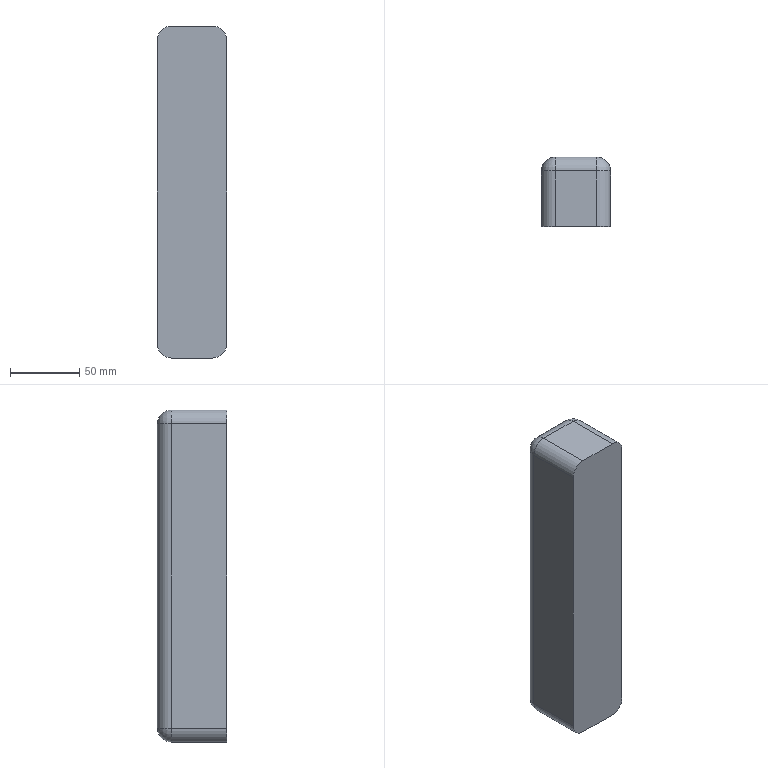Part | SolidWorks | features ICE 2, Extrusion 1, Fillet 1 | 1 solid | 18 faces | box 50 x 50 x 240 mm | volume 583931 mm3 | cylinder 8 | plane 6 | sphere 4 | commonest cylinder face diameters 20 x8
STEP:
#1=CARTESIAN_POINT('',(0.,40.,10.));
#2=VERTEX_POINT('',#1);
#3=CARTESIAN_POINT('',(0.,0.,10.));
#4=VERTEX_POINT('',#3);
#5=CARTESIAN_POINT('',(0.,0.,10.));
#6=DIRECTION('',(0.,-1.,0.));
#7=VECTOR('',#6,1000.);
#8=LINE('',#5,#7);
#9=EDGE_CURVE('',#2,#4,#8,.T.);
#10=ORIENTED_EDGE('',*,*,#9,.T.);
#11=CARTESIAN_POINT('',(0.,0.,230.));
#12=VERTEX_POINT('',#11);
#13=CARTESIAN_POINT('',(0.,0.,290.));
#14=DIRECTION('',(0.,0.,-1.));
#15=VECTOR('',#14,1000.);
#16=LINE('',#13,#15);
#17=EDGE_CURVE('',#12,#4,#16,.T.);
#18=ORIENTED_EDGE('',*,*,#17,.F.);
#19=CARTESIAN_POINT('',(0.,40.,230.));
#20=VERTEX_POINT('',#19);
#21=CARTESIAN_POINT('',(0.,50.,230.));
#22=DIRECTION('',(0.,1.,0.));
#23=VECTOR('',#22,1000.);
#24=LINE('',#21,#23);
#25=EDGE_CURVE('',#12,#20,#24,.T.);
#26=ORIENTED_EDGE('',*,*,#25,.T.);
#27=CARTESIAN_POINT('',(0.,40.,240.));
#28=DIRECTION('',(0.,0.,-1.));
#29=VECTOR('',#28,1000.);
#30=LINE('',#27,#29);
#31=EDGE_CURVE('',#20,#2,#30,.T.);
#32=ORIENTED_EDGE('',*,*,#31,.T.);
#33=EDGE_LOOP('',(#10,#18,#26,#32));
#34=FACE_OUTER_BOUND('',#33,.T.);
#35=CARTESIAN_POINT('',(0.,0.,240.));
#36=DIRECTION('',(1.,0.,0.));
#37=DIRECTION('',(0.,0.,-1.));
#38=AXIS2_PLACEMENT_3D('',#35,#36,#37);
#39=PLANE('',#38);
#40=ADVANCED_FACE('',(#34),#39,.F.);
#41=CARTESIAN_POINT('',(50.,40.,230.));
#42=VERTEX_POINT('',#41);
#43=CARTESIAN_POINT('',(50.,0.,230.));
#44=VERTEX_POINT('',#43);
#45=CARTESIAN_POINT('',(50.,0.,230.));
#46=DIRECTION('',(0.,-1.,0.));
#47=VECTOR('',#46,1000.);
#48=LINE('',#45,#47);
#49=EDGE_CURVE('',#42,#44,#48,.T.);
#50=ORIENTED_EDGE('',*,*,#49,.T.);
#51=CARTESIAN_POINT('',(50.,0.,10.));
#52=VERTEX_POINT('',#51);
#53=CARTESIAN_POINT('',(50.,0.,240.));
#54=DIRECTION('',(0.,0.,-1.));
#55=VECTOR('',#54,1000.);
#56=LINE('',#53,#55);
#57=EDGE_CURVE('',#44,#52,#56,.T.);
#58=ORIENTED_EDGE('',*,*,#57,.T.);
#59=CARTESIAN_POINT('',(50.,40.,10.));
#60=VERTEX_POINT('',#59);
#61=CARTESIAN_POINT('',(50.,0.,10.));
#62=DIRECTION('',(0.,1.,0.));
#63=VECTOR('',#62,1000.);
#64=LINE('',#61,#63);
#65=EDGE_CURVE('',#52,#60,#64,.T.);
#66=ORIENTED_EDGE('',*,*,#65,.T.);
#67=CARTESIAN_POINT('',(50.,40.,240.));
#68=DIRECTION('',(0.,0.,1.));
#69=VECTOR('',#68,1000.);
#70=LINE('',#67,#69);
#71=EDGE_CURVE('',#60,#42,#70,.T.);
#72=ORIENTED_EDGE('',*,*,#71,.T.);
#73=EDGE_LOOP('',(#50,#58,#66,#72));
#74=FACE_OUTER_BOUND('',#73,.T.);
#75=CARTESIAN_POINT('',(50.,0.,240.));
#76=DIRECTION('',(-1.,0.,0.));
#77=DIRECTION('',(0.,0.,1.));
#78=AXIS2_PLACEMENT_3D('',#75,#76,#77);
#79=PLANE('',#78);
#80=ADVANCED_FACE('',(#74),#79,.F.);
#81=CARTESIAN_POINT('',(10.,50.,10.));
#82=VERTEX_POINT('',#81);
#83=CARTESIAN_POINT('',(10.,50.,230.));
#84=VERTEX_POINT('',#83);
#85=CARTESIAN_POINT('',(10.,50.,240.));
#86=DIRECTION('',(0.,0.,1.));
#87=VECTOR('',#86,1000.);
#88=LINE('',#85,#87);
#89=EDGE_CURVE('',#82,#84,#88,.T.);
#90=ORIENTED_EDGE('',*,*,#89,.T.);
#91=CARTESIAN_POINT('',(40.,50.,230.));
#92=VERTEX_POINT('',#91);
#93=CARTESIAN_POINT('',(50.,50.,230.));
#94=DIRECTION('',(1.,0.,0.));
#95=VECTOR('',#94,1000.);
#96=LINE('',#93,#95);
#97=EDGE_CURVE('',#84,#92,#96,.T.);
#98=ORIENTED_EDGE('',*,*,#97,.T.);
#99=CARTESIAN_POINT('',(40.,50.,10.));
#100=VERTEX_POINT('',#99);
#101=CARTESIAN_POINT('',(40.,50.,240.));
#102=DIRECTION('',(0.,0.,-1.));
#103=VECTOR('',#102,1000.);
#104=LINE('',#101,#103);
#105=EDGE_CURVE('',#92,#100,#104,.T.);
#106=ORIENTED_EDGE('',*,*,#105,.T.);
#107=CARTESIAN_POINT('',(50.,50.,10.));
#108=DIRECTION('',(-1.,0.,0.));
#109=VECTOR('',#108,1000.);
#110=LINE('',#107,#109);
#111=EDGE_CURVE('',#100,#82,#110,.T.);
#112=ORIENTED_EDGE('',*,*,#111,.T.);
#113=EDGE_LOOP('',(#90,#98,#106,#112));
#114=FACE_OUTER_BOUND('',#113,.T.);
#115=CARTESIAN_POINT('',(50.,50.,240.));
#116=DIRECTION('',(0.,-1.,0.));
#117=DIRECTION('',(0.,0.,-1.));
#118=AXIS2_PLACEMENT_3D('',#115,#116,#117);
#119=PLANE('',#118);
#120=ADVANCED_FACE('',(#114),#119,.F.);
#121=CARTESIAN_POINT('',(40.,40.,240.));
#122=VERTEX_POINT('',#121);
#123=CARTESIAN_POINT('',(10.,40.,240.));
#124=VERTEX_POINT('',#123);
#125=CARTESIAN_POINT('',(0.,40.,240.));
#126=DIRECTION('',(-1.,0.,0.));
#127=VECTOR('',#126,1000.);
#128=LINE('',#125,#127);
#129=EDGE_CURVE('',#122,#124,#128,.T.);
#130=ORIENTED_EDGE('',*,*,#129,.T.);
#131=CARTESIAN_POINT('',(10.,0.,240.));
#132=VERTEX_POINT('',#131);
#133=CARTESIAN_POINT('',(10.,0.,240.));
#134=DIRECTION('',(0.,-1.,0.));
#135=VECTOR('',#134,1000.);
#136=LINE('',#133,#135);
#137=EDGE_CURVE('',#124,#132,#136,.T.);
#138=ORIENTED_EDGE('',*,*,#137,.T.);
#139=CARTESIAN_POINT('',(40.,0.,240.));
#140=VERTEX_POINT('',#139);
#141=CARTESIAN_POINT('',(0.,0.,240.));
#142=DIRECTION('',(1.,0.,0.));
#143=VECTOR('',#142,1000.);
#144=LINE('',#141,#143);
#145=EDGE_CURVE('',#132,#140,#144,.T.);
#146=ORIENTED_EDGE('',*,*,#145,.T.);
#147=CARTESIAN_POINT('',(40.,50.,240.));
#148=DIRECTION('',(0.,1.,0.));
#149=VECTOR('',#148,1000.);
#150=LINE('',#147,#149);
#151=EDGE_CURVE('',#140,#122,#150,.T.);
#152=ORIENTED_EDGE('',*,*,#151,.T.);
#153=EDGE_LOOP('',(#130,#138,#146,#152));
#154=FACE_OUTER_BOUND('',#153,.T.);
#155=CARTESIAN_POINT('',(0.,0.,240.));
#156=DIRECTION('',(0.,0.,1.));
#157=DIRECTION('',(1.,0.,0.));
#158=AXIS2_PLACEMENT_3D('',#155,#156,#157);
#159=PLANE('',#158);
#160=ADVANCED_FACE('',(#154),#159,.T.);
#161=CARTESIAN_POINT('',(10.,40.,0.));
#162=VERTEX_POINT('',#161);
#163=CARTESIAN_POINT('',(40.,40.,0.));
#164=VERTEX_POINT('',#163);
#165=CARTESIAN_POINT('',(0.,40.,0.));
#166=DIRECTION('',(1.,0.,0.));
#167=VECTOR('',#166,1000.);
#168=LINE('',#165,#167);
#169=EDGE_CURVE('',#162,#164,#168,.T.);
#170=ORIENTED_EDGE('',*,*,#169,.T.);
#171=CARTESIAN_POINT('',(40.,0.,0.));
#172=VERTEX_POINT('',#171);
#173=CARTESIAN_POINT('',(40.,0.,0.));
#174=DIRECTION('',(0.,-1.,0.));
#175=VECTOR('',#174,1000.);
#176=LINE('',#173,#175);
#177=EDGE_CURVE('',#164,#172,#176,.T.);
#178=ORIENTED_EDGE('',*,*,#177,.T.);
#179=CARTESIAN_POINT('',(10.,0.,0.));
#180=VERTEX_POINT('',#179);
#181=CARTESIAN_POINT('',(0.,0.,0.));
#182=DIRECTION('',(1.,0.,0.));
#183=VECTOR('',#182,1000.);
#184=LINE('',#181,#183);
#185=EDGE_CURVE('',#180,#172,#184,.T.);
#186=ORIENTED_EDGE('',*,*,#185,.F.);
#187=CARTESIAN_POINT('',(10.,0.,0.));
#188=DIRECTION('',(0.,1.,0.));
#189=VECTOR('',#188,1000.);
#190=LINE('',#187,#189);
#191=EDGE_CURVE('',#180,#162,#190,.T.);
#192=ORIENTED_EDGE('',*,*,#191,.T.);
#193=EDGE_LOOP('',(#170,#178,#186,#192));
#194=FACE_OUTER_BOUND('',#193,.T.);
#195=CARTESIAN_POINT('',(0.,0.,0.));
#196=DIRECTION('',(0.,0.,1.));
#197=DIRECTION('',(1.,0.,0.));
#198=AXIS2_PLACEMENT_3D('',#195,#196,#197);
#199=PLANE('',#198);
#200=ADVANCED_FACE('',(#194),#199,.F.);
#201=CARTESIAN_POINT('',(40.,0.,10.));
#202=DIRECTION('',(0.,-1.,0.));
#203=DIRECTION('',(0.,0.,1.));
#204=AXIS2_PLACEMENT_3D('',#201,#202,#203);
#205=CIRCLE('',#204,10.);
#206=EDGE_CURVE('',#172,#52,#205,.T.);
#207=ORIENTED_EDGE('',*,*,#206,.F.);
#208=ORIENTED_EDGE('',*,*,#177,.F.);
#209=CARTESIAN_POINT('',(40.,40.,10.));
#210=DIRECTION('',(0.,1.,0.));
#211=DIRECTION('',(0.,0.,1.));
#212=AXIS2_PLACEMENT_3D('',#209,#210,#211);
#213=CIRCLE('',#212,10.);
#214=EDGE_CURVE('',#60,#164,#213,.T.);
#215=ORIENTED_EDGE('',*,*,#214,.F.);
#216=ORIENTED_EDGE('',*,*,#65,.F.);
#217=EDGE_LOOP('',(#207,#208,#215,#216));
#218=FACE_OUTER_BOUND('',#217,.T.);
#219=CARTESIAN_POINT('',(40.,0.,10.));
#220=DIRECTION('',(0.,1.,0.));
#221=DIRECTION('',(0.,0.,1.));
#222=AXIS2_PLACEMENT_3D('',#219,#220,#221);
#223=CYLINDRICAL_SURFACE('',#222,10.);
#224=ADVANCED_FACE('',(#218),#223,.T.);
#225=CARTESIAN_POINT('',(10.,0.,10.));
#226=DIRECTION('',(0.,-1.,0.));
#227=DIRECTION('',(0.,0.,1.));
#228=AXIS2_PLACEMENT_3D('',#225,#226,#227);
#229=CIRCLE('',#228,10.);
#230=EDGE_CURVE('',#4,#180,#229,.T.);
#231=ORIENTED_EDGE('',*,*,#230,.F.);
#232=ORIENTED_EDGE('',*,*,#9,.F.);
#233=CARTESIAN_POINT('',(10.,40.,10.));
#234=DIRECTION('',(0.,1.,0.));
#235=DIRECTION('',(0.,0.,1.));
#236=AXIS2_PLACEMENT_3D('',#233,#234,#235);
#237=CIRCLE('',#236,10.);
#238=EDGE_CURVE('',#162,#2,#237,.T.);
#239=ORIENTED_EDGE('',*,*,#238,.F.);
#240=ORIENTED_EDGE('',*,*,#191,.F.);
#241=EDGE_LOOP('',(#231,#232,#239,#240));
#242=FACE_OUTER_BOUND('',#241,.T.);
#243=CARTESIAN_POINT('',(10.,0.,10.));
#244=DIRECTION('',(0.,-1.,0.));
#245=DIRECTION('',(0.,0.,-1.));
#246=AXIS2_PLACEMENT_3D('',#243,#244,#245);
#247=CYLINDRICAL_SURFACE('',#246,10.);
#248=ADVANCED_FACE('',(#242),#247,.T.);
#249=CARTESIAN_POINT('',(40.,40.,10.));
#250=DIRECTION('',(1.,0.,0.));
#251=DIRECTION('',(0.,0.,-1.));
#252=AXIS2_PLACEMENT_3D('',#249,#250,#251);
#253=CIRCLE('',#252,10.);
#254=EDGE_CURVE('',#164,#100,#253,.T.);
#255=ORIENTED_EDGE('',*,*,#254,.F.);
#256=ORIENTED_EDGE('',*,*,#169,.F.);
#257=CARTESIAN_POINT('',(10.,40.,10.));
#258=DIRECTION('',(-1.,0.,0.));
#259=DIRECTION('',(0.,0.,1.));
#260=AXIS2_PLACEMENT_3D('',#257,#258,#259);
#261=CIRCLE('',#260,10.);
#262=EDGE_CURVE('',#82,#162,#261,.T.);
#263=ORIENTED_EDGE('',*,*,#262,.F.);
#264=ORIENTED_EDGE('',*,*,#111,.F.);
#265=EDGE_LOOP('',(#255,#256,#263,#264));
#266=FACE_OUTER_BOUND('',#265,.T.);
#267=CARTESIAN_POINT('',(50.,40.,10.));
#268=DIRECTION('',(-1.,0.,0.));
#269=DIRECTION('',(0.,0.,1.));
#270=AXIS2_PLACEMENT_3D('',#267,#268,#269);
#271=CYLINDRICAL_SURFACE('',#270,10.);
#272=ADVANCED_FACE('',(#266),#271,.T.);
#273=ORIENTED_EDGE('',*,*,#214,.T.);
#274=ORIENTED_EDGE('',*,*,#254,.T.);
#275=CARTESIAN_POINT('',(40.,40.,10.));
#276=DIRECTION('',(0.,0.,1.));
#277=DIRECTION('',(-1.,0.,0.));
#278=AXIS2_PLACEMENT_3D('',#275,#276,#277);
#279=CIRCLE('',#278,10.);
#280=EDGE_CURVE('',#60,#100,#279,.T.);
#281=ORIENTED_EDGE('',*,*,#280,.F.);
#282=EDGE_LOOP('',(#273,#274,#281));
#283=FACE_OUTER_BOUND('',#282,.T.);
#284=CARTESIAN_POINT('',(40.,40.,10.));
#285=DIRECTION('',(0.,1.,0.));
#286=DIRECTION('',(1.,0.,0.));
#287=AXIS2_PLACEMENT_3D('',#284,#285,#286);
#288=SPHERICAL_SURFACE('',#287,10.);
#289=ADVANCED_FACE('',(#283),#288,.T.);
#290=ORIENTED_EDGE('',*,*,#262,.T.);
#291=ORIENTED_EDGE('',*,*,#238,.T.);
#292=CARTESIAN_POINT('',(10.,40.,10.));
#293=DIRECTION('',(0.,0.,1.));
#294=DIRECTION('',(-1.,0.,0.));
#295=AXIS2_PLACEMENT_3D('',#292,#293,#294);
#296=CIRCLE('',#295,10.);
#297=EDGE_CURVE('',#82,#2,#296,.T.);
#298=ORIENTED_EDGE('',*,*,#297,.F.);
#299=EDGE_LOOP('',(#290,#291,#298));
#300=FACE_OUTER_BOUND('',#299,.T.);
#301=CARTESIAN_POINT('',(10.,40.,10.));
#302=DIRECTION('',(0.,1.,0.));
#303=DIRECTION('',(1.,0.,0.));
#304=AXIS2_PLACEMENT_3D('',#301,#302,#303);
#305=SPHERICAL_SURFACE('',#304,10.);
#306=ADVANCED_FACE('',(#300),#305,.T.);
#307=ORIENTED_EDGE('',*,*,#280,.T.);
#308=ORIENTED_EDGE('',*,*,#105,.F.);
#309=CARTESIAN_POINT('',(40.,40.,230.));
#310=DIRECTION('',(0.,0.,1.));
#311=DIRECTION('',(1.,0.,0.));
#312=AXIS2_PLACEMENT_3D('',#309,#310,#311);
#313=CIRCLE('',#312,10.);
#314=EDGE_CURVE('',#42,#92,#313,.T.);
#315=ORIENTED_EDGE('',*,*,#314,.F.);
#316=ORIENTED_EDGE('',*,*,#71,.F.);
#317=EDGE_LOOP('',(#307,#308,#315,#316));
#318=FACE_OUTER_BOUND('',#317,.T.);
#319=CARTESIAN_POINT('',(40.,40.,240.));
#320=DIRECTION('',(0.,0.,-1.));
#321=DIRECTION('',(-1.,0.,0.));
#322=AXIS2_PLACEMENT_3D('',#319,#320,#321);
#323=CYLINDRICAL_SURFACE('',#322,10.);
#324=ADVANCED_FACE('',(#318),#323,.T.);
#325=CARTESIAN_POINT('',(40.,0.,230.));
#326=DIRECTION('',(0.,-1.,0.));
#327=DIRECTION('',(0.,0.,1.));
#328=AXIS2_PLACEMENT_3D('',#325,#326,#327);
#329=CIRCLE('',#328,10.);
#330=EDGE_CURVE('',#44,#140,#329,.T.);
#331=ORIENTED_EDGE('',*,*,#330,.F.);
#332=ORIENTED_EDGE('',*,*,#49,.F.);
#333=CARTESIAN_POINT('',(40.,40.,230.));
#334=DIRECTION('',(0.,1.,0.));
#335=DIRECTION('',(0.,0.,1.));
#336=AXIS2_PLACEMENT_3D('',#333,#334,#335);
#337=CIRCLE('',#336,10.);
#338=EDGE_CURVE('',#122,#42,#337,.T.);
#339=ORIENTED_EDGE('',*,*,#338,.F.);
#340=ORIENTED_EDGE('',*,*,#151,.F.);
#341=EDGE_LOOP('',(#331,#332,#339,#340));
#342=FACE_OUTER_BOUND('',#341,.T.);
#343=CARTESIAN_POINT('',(40.,0.,230.));
#344=DIRECTION('',(0.,-1.,0.));
#345=DIRECTION('',(0.,0.,-1.));
#346=AXIS2_PLACEMENT_3D('',#343,#344,#345);
#347=CYLINDRICAL_SURFACE('',#346,10.);
#348=ADVANCED_FACE('',(#342),#347,.T.);
#349=CARTESIAN_POINT('',(10.,0.,230.));
#350=DIRECTION('',(0.,-1.,0.));
#351=DIRECTION('',(0.,0.,1.));
#352=AXIS2_PLACEMENT_3D('',#349,#350,#351);
#353=CIRCLE('',#352,10.);
#354=EDGE_CURVE('',#132,#12,#353,.T.);
#355=ORIENTED_EDGE('',*,*,#354,.F.);
#356=ORIENTED_EDGE('',*,*,#137,.F.);
#357=CARTESIAN_POINT('',(10.,40.,230.));
#358=DIRECTION('',(0.,1.,0.));
#359=DIRECTION('',(0.,0.,1.));
#360=AXIS2_PLACEMENT_3D('',#357,#358,#359);
#361=CIRCLE('',#360,10.);
#362=EDGE_CURVE('',#20,#124,#361,.T.);
#363=ORIENTED_EDGE('',*,*,#362,.F.);
#364=ORIENTED_EDGE('',*,*,#25,.F.);
#365=EDGE_LOOP('',(#355,#356,#363,#364));
#366=FACE_OUTER_BOUND('',#365,.T.);
#367=CARTESIAN_POINT('',(10.,0.,230.));
#368=DIRECTION('',(0.,1.,0.));
#369=DIRECTION('',(0.,0.,1.));
#370=AXIS2_PLACEMENT_3D('',#367,#368,#369);
#371=CYLINDRICAL_SURFACE('',#370,10.);
#372=ADVANCED_FACE('',(#366),#371,.T.);
#373=ORIENTED_EDGE('',*,*,#297,.T.);
#374=ORIENTED_EDGE('',*,*,#31,.F.);
#375=CARTESIAN_POINT('',(10.,40.,230.));
#376=DIRECTION('',(0.,0.,1.));
#377=DIRECTION('',(1.,0.,0.));
#378=AXIS2_PLACEMENT_3D('',#375,#376,#377);
#379=CIRCLE('',#378,10.);
#380=EDGE_CURVE('',#84,#20,#379,.T.);
#381=ORIENTED_EDGE('',*,*,#380,.F.);
#382=ORIENTED_EDGE('',*,*,#89,.F.);
#383=EDGE_LOOP('',(#373,#374,#381,#382));
#384=FACE_OUTER_BOUND('',#383,.T.);
#385=CARTESIAN_POINT('',(10.,40.,240.));
#386=DIRECTION('',(0.,0.,-1.));
#387=DIRECTION('',(-1.,0.,0.));
#388=AXIS2_PLACEMENT_3D('',#385,#386,#387);
#389=CYLINDRICAL_SURFACE('',#388,10.);
#390=ADVANCED_FACE('',(#384),#389,.T.);
#391=ORIENTED_EDGE('',*,*,#338,.T.);
#392=ORIENTED_EDGE('',*,*,#314,.T.);
#393=CARTESIAN_POINT('',(40.,40.,230.));
#394=DIRECTION('',(-1.,0.,0.));
#395=DIRECTION('',(0.,0.,-1.));
#396=AXIS2_PLACEMENT_3D('',#393,#394,#395);
#397=CIRCLE('',#396,10.);
#398=EDGE_CURVE('',#122,#92,#397,.T.);
#399=ORIENTED_EDGE('',*,*,#398,.F.);
#400=EDGE_LOOP('',(#391,#392,#399));
#401=FACE_OUTER_BOUND('',#400,.T.);
#402=CARTESIAN_POINT('',(40.,40.,230.));
#403=DIRECTION('',(0.,1.,0.));
#404=DIRECTION('',(1.,0.,0.));
#405=AXIS2_PLACEMENT_3D('',#402,#403,#404);
#406=SPHERICAL_SURFACE('',#405,10.);
#407=ADVANCED_FACE('',(#401),#406,.T.);
#408=ORIENTED_EDGE('',*,*,#380,.T.);
#409=ORIENTED_EDGE('',*,*,#362,.T.);
#410=CARTESIAN_POINT('',(10.,40.,230.));
#411=DIRECTION('',(1.,0.,0.));
#412=DIRECTION('',(0.,0.,1.));
#413=AXIS2_PLACEMENT_3D('',#410,#411,#412);
#414=CIRCLE('',#413,10.);
#415=EDGE_CURVE('',#84,#124,#414,.T.);
#416=ORIENTED_EDGE('',*,*,#415,.F.);
#417=EDGE_LOOP('',(#408,#409,#416));
#418=FACE_OUTER_BOUND('',#417,.T.);
#419=CARTESIAN_POINT('',(10.,40.,230.));
#420=DIRECTION('',(0.,1.,0.));
#421=DIRECTION('',(1.,0.,0.));
#422=AXIS2_PLACEMENT_3D('',#419,#420,#421);
#423=SPHERICAL_SURFACE('',#422,10.);
#424=ADVANCED_FACE('',(#418),#423,.T.);
#425=ORIENTED_EDGE('',*,*,#398,.T.);
#426=ORIENTED_EDGE('',*,*,#97,.F.);
#427=ORIENTED_EDGE('',*,*,#415,.T.);
#428=ORIENTED_EDGE('',*,*,#129,.F.);
#429=EDGE_LOOP('',(#425,#426,#427,#428));
#430=FACE_OUTER_BOUND('',#429,.T.);
#431=CARTESIAN_POINT('',(0.,40.,230.));
#432=DIRECTION('',(1.,0.,0.));
#433=DIRECTION('',(0.,0.,-1.));
#434=AXIS2_PLACEMENT_3D('',#431,#432,#433);
#435=CYLINDRICAL_SURFACE('',#434,10.);
#436=ADVANCED_FACE('',(#430),#435,.T.);
#437=ORIENTED_EDGE('',*,*,#230,.T.);
#438=ORIENTED_EDGE('',*,*,#185,.T.);
#439=ORIENTED_EDGE('',*,*,#206,.T.);
#440=ORIENTED_EDGE('',*,*,#57,.F.);
#441=ORIENTED_EDGE('',*,*,#330,.T.);
#442=ORIENTED_EDGE('',*,*,#145,.F.);
#443=ORIENTED_EDGE('',*,*,#354,.T.);
#444=ORIENTED_EDGE('',*,*,#17,.T.);
#445=EDGE_LOOP('',(#437,#438,#439,#440,#441,#442,#443,#444));
#446=FACE_OUTER_BOUND('',#445,.T.);
#447=CARTESIAN_POINT('',(59.,0.,290.));
#448=DIRECTION('',(0.,1.,0.));
#449=DIRECTION('',(0.,0.,1.));
#450=AXIS2_PLACEMENT_3D('',#447,#448,#449);
#451=PLANE('',#450);
#452=ADVANCED_FACE('',(#446),#451,.F.);
#453=CLOSED_SHELL('',(#40,#80,#120,#160,#200,#224,#248,#272,#289,#306,#324,#348,#372,#390,#407,#424,#436,#452));
#454=MANIFOLD_SOLID_BREP('',#453);
#455=CARTESIAN_POINT('',(0.,0.,0.));
#456=DIRECTION('',(0.,0.,1.));
#457=DIRECTION('',(1.,0.,0.));
#458=AXIS2_PLACEMENT_3D('',#455,#456,#457);
#459=(LENGTH_UNIT()NAMED_UNIT(*)SI_UNIT(.MILLI.,.METRE.));
#460=UNCERTAINTY_MEASURE_WITH_UNIT(LENGTH_MEASURE(0.00001),#459,'','');
#461=(NAMED_UNIT(*)PLANE_ANGLE_UNIT()SI_UNIT($,.RADIAN.));
#462=(NAMED_UNIT(*)SI_UNIT($,.STERADIAN.)SOLID_ANGLE_UNIT());
#463=(GEOMETRIC_REPRESENTATION_CONTEXT(3)GLOBAL_UNCERTAINTY_ASSIGNED_CONTEXT((#460))GLOBAL_UNIT_ASSIGNED_CONTEXT((#459,#461,#462))REPRESENTATION_CONTEXT('',''));
#464=ADVANCED_BREP_SHAPE_REPRESENTATION('',(#454,#458),#463);